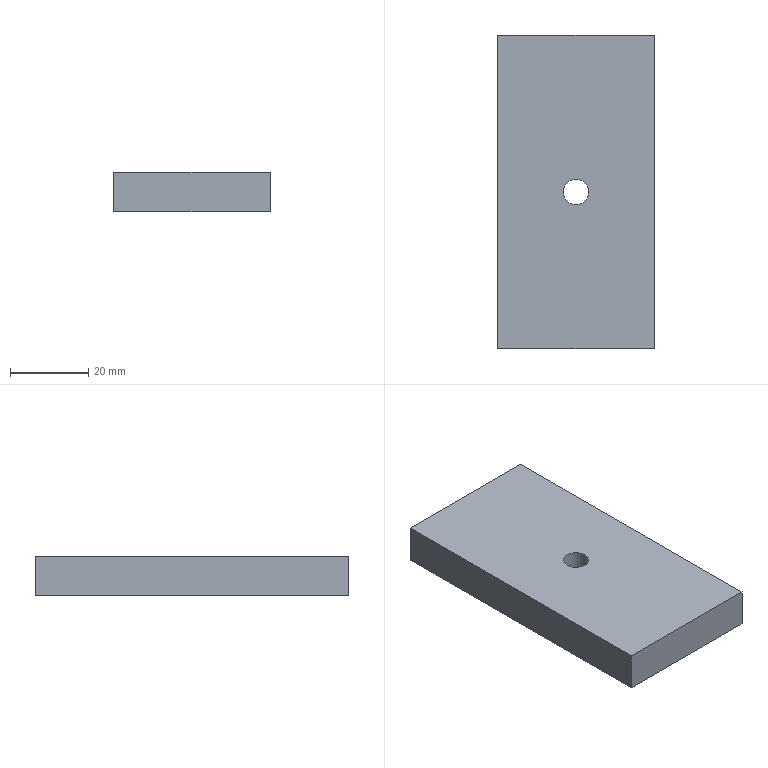Part | STEP file | SynoNew-0304-045 | 1 solid | 7 faces | box 40 x 80 x 10 mm | volume 31668 mm3 | plane 6 | cylinder 1 | commonest cylinder face diameters 6.5 x1
STEP:
#1=CARTESIAN_POINT('',(3.25,0.,10.));
#2=VERTEX_POINT('',#1);
#3=CARTESIAN_POINT('',(-3.25,0.,10.));
#4=VERTEX_POINT('',#3);
#5=CARTESIAN_POINT('',(0.,0.,10.));
#6=DIRECTION('',(0.,0.,-1.));
#7=DIRECTION('',(1.,0.,0.));
#8=AXIS2_PLACEMENT_3D('',#5,#6,#7);
#9=CIRCLE('',#8,3.25);
#10=EDGE_CURVE('',#2,#4,#9,.T.);
#11=ORIENTED_EDGE('',*,*,#10,.F.);
#12=CARTESIAN_POINT('',(0.,0.,10.));
#13=DIRECTION('',(0.,0.,-1.));
#14=DIRECTION('',(1.,0.,0.));
#15=AXIS2_PLACEMENT_3D('',#12,#13,#14);
#16=CIRCLE('',#15,3.25);
#17=EDGE_CURVE('',#4,#2,#16,.T.);
#18=ORIENTED_EDGE('',*,*,#17,.F.);
#19=CARTESIAN_POINT('',(-3.25,0.,0.));
#20=VERTEX_POINT('',#19);
#21=CARTESIAN_POINT('',(-3.25,0.,-80.));
#22=DIRECTION('',(0.,0.,-1.));
#23=VECTOR('',#22,3.25);
#24=LINE('',#21,#23);
#25=EDGE_CURVE('',#4,#20,#24,.T.);
#26=ORIENTED_EDGE('',*,*,#25,.T.);
#27=CARTESIAN_POINT('',(0.,0.,0.));
#28=DIRECTION('',(0.,0.,1.));
#29=DIRECTION('',(1.,0.,0.));
#30=AXIS2_PLACEMENT_3D('',#27,#28,#29);
#31=CIRCLE('',#30,3.25);
#32=EDGE_CURVE('',#20,#20,#31,.T.);
#33=ORIENTED_EDGE('',*,*,#32,.F.);
#34=ORIENTED_EDGE('',*,*,#25,.F.);
#35=EDGE_LOOP('',(#11,#18,#26,#33,#34));
#36=FACE_OUTER_BOUND('',#35,.T.);
#37=CARTESIAN_POINT('',(0.,0.,-80.));
#38=DIRECTION('',(0.,0.,1.));
#39=DIRECTION('',(1.,0.,0.));
#40=AXIS2_PLACEMENT_3D('',#37,#38,#39);
#41=CYLINDRICAL_SURFACE('',#40,3.25);
#42=ADVANCED_FACE('',(#36),#41,.F.);
#43=CARTESIAN_POINT('',(-20.,-40.,0.));
#44=VERTEX_POINT('',#43);
#45=CARTESIAN_POINT('',(20.,-40.,0.));
#46=VERTEX_POINT('',#45);
#47=CARTESIAN_POINT('',(-20.,-40.,0.));
#48=DIRECTION('',(1.,0.,0.));
#49=VECTOR('',#48,10.);
#50=LINE('',#47,#49);
#51=EDGE_CURVE('',#44,#46,#50,.T.);
#52=ORIENTED_EDGE('',*,*,#51,.T.);
#53=CARTESIAN_POINT('',(20.,-40.,10.));
#54=VERTEX_POINT('',#53);
#55=CARTESIAN_POINT('',(20.,-40.,0.));
#56=DIRECTION('',(0.,0.,1.));
#57=VECTOR('',#56,10.);
#58=LINE('',#55,#57);
#59=EDGE_CURVE('',#46,#54,#58,.T.);
#60=ORIENTED_EDGE('',*,*,#59,.T.);
#61=CARTESIAN_POINT('',(-20.,-40.,10.));
#62=VERTEX_POINT('',#61);
#63=CARTESIAN_POINT('',(-20.,-40.,10.));
#64=DIRECTION('',(1.,0.,0.));
#65=VECTOR('',#64,10.);
#66=LINE('',#63,#65);
#67=EDGE_CURVE('',#62,#54,#66,.T.);
#68=ORIENTED_EDGE('',*,*,#67,.F.);
#69=CARTESIAN_POINT('',(-20.,-40.,0.));
#70=DIRECTION('',(0.,0.,1.));
#71=VECTOR('',#70,10.);
#72=LINE('',#69,#71);
#73=EDGE_CURVE('',#44,#62,#72,.T.);
#74=ORIENTED_EDGE('',*,*,#73,.F.);
#75=EDGE_LOOP('',(#52,#60,#68,#74));
#76=FACE_OUTER_BOUND('',#75,.T.);
#77=CARTESIAN_POINT('',(-20.,-40.,0.));
#78=DIRECTION('',(0.,-1.,0.));
#79=DIRECTION('',(1.,0.,0.));
#80=AXIS2_PLACEMENT_3D('',#77,#78,#79);
#81=PLANE('',#80);
#82=ADVANCED_FACE('',(#76),#81,.T.);
#83=CARTESIAN_POINT('',(-20.,40.,0.));
#84=VERTEX_POINT('',#83);
#85=CARTESIAN_POINT('',(-20.,40.,0.));
#86=DIRECTION('',(0.,-1.,0.));
#87=VECTOR('',#86,10.);
#88=LINE('',#85,#87);
#89=EDGE_CURVE('',#84,#44,#88,.T.);
#90=ORIENTED_EDGE('',*,*,#89,.T.);
#91=ORIENTED_EDGE('',*,*,#73,.T.);
#92=CARTESIAN_POINT('',(-20.,40.,10.));
#93=VERTEX_POINT('',#92);
#94=CARTESIAN_POINT('',(-20.,40.,10.));
#95=DIRECTION('',(0.,-1.,0.));
#96=VECTOR('',#95,10.);
#97=LINE('',#94,#96);
#98=EDGE_CURVE('',#93,#62,#97,.T.);
#99=ORIENTED_EDGE('',*,*,#98,.F.);
#100=CARTESIAN_POINT('',(-20.,40.,0.));
#101=DIRECTION('',(0.,0.,1.));
#102=VECTOR('',#101,10.);
#103=LINE('',#100,#102);
#104=EDGE_CURVE('',#84,#93,#103,.T.);
#105=ORIENTED_EDGE('',*,*,#104,.F.);
#106=EDGE_LOOP('',(#90,#91,#99,#105));
#107=FACE_OUTER_BOUND('',#106,.T.);
#108=CARTESIAN_POINT('',(-20.,40.,0.));
#109=DIRECTION('',(-1.,0.,0.));
#110=DIRECTION('',(0.,-1.,0.));
#111=AXIS2_PLACEMENT_3D('',#108,#109,#110);
#112=PLANE('',#111);
#113=ADVANCED_FACE('',(#107),#112,.T.);
#114=CARTESIAN_POINT('',(20.,40.,0.));
#115=VERTEX_POINT('',#114);
#116=CARTESIAN_POINT('',(20.,40.,0.));
#117=DIRECTION('',(-1.,0.,0.));
#118=VECTOR('',#117,10.);
#119=LINE('',#116,#118);
#120=EDGE_CURVE('',#115,#84,#119,.T.);
#121=ORIENTED_EDGE('',*,*,#120,.T.);
#122=ORIENTED_EDGE('',*,*,#104,.T.);
#123=CARTESIAN_POINT('',(20.,40.,10.));
#124=VERTEX_POINT('',#123);
#125=CARTESIAN_POINT('',(20.,40.,10.));
#126=DIRECTION('',(-1.,0.,0.));
#127=VECTOR('',#126,10.);
#128=LINE('',#125,#127);
#129=EDGE_CURVE('',#124,#93,#128,.T.);
#130=ORIENTED_EDGE('',*,*,#129,.F.);
#131=CARTESIAN_POINT('',(20.,40.,0.));
#132=DIRECTION('',(0.,0.,1.));
#133=VECTOR('',#132,10.);
#134=LINE('',#131,#133);
#135=EDGE_CURVE('',#115,#124,#134,.T.);
#136=ORIENTED_EDGE('',*,*,#135,.F.);
#137=EDGE_LOOP('',(#121,#122,#130,#136));
#138=FACE_OUTER_BOUND('',#137,.T.);
#139=CARTESIAN_POINT('',(20.,40.,0.));
#140=DIRECTION('',(0.,1.,0.));
#141=DIRECTION('',(-1.,0.,0.));
#142=AXIS2_PLACEMENT_3D('',#139,#140,#141);
#143=PLANE('',#142);
#144=ADVANCED_FACE('',(#138),#143,.T.);
#145=CARTESIAN_POINT('',(20.,-40.,0.));
#146=DIRECTION('',(0.,1.,0.));
#147=VECTOR('',#146,10.);
#148=LINE('',#145,#147);
#149=EDGE_CURVE('',#46,#115,#148,.T.);
#150=ORIENTED_EDGE('',*,*,#149,.T.);
#151=ORIENTED_EDGE('',*,*,#135,.T.);
#152=CARTESIAN_POINT('',(20.,-40.,10.));
#153=DIRECTION('',(0.,1.,0.));
#154=VECTOR('',#153,10.);
#155=LINE('',#152,#154);
#156=EDGE_CURVE('',#54,#124,#155,.T.);
#157=ORIENTED_EDGE('',*,*,#156,.F.);
#158=ORIENTED_EDGE('',*,*,#59,.F.);
#159=EDGE_LOOP('',(#150,#151,#157,#158));
#160=FACE_OUTER_BOUND('',#159,.T.);
#161=CARTESIAN_POINT('',(20.,-40.,0.));
#162=DIRECTION('',(1.,0.,0.));
#163=DIRECTION('',(0.,1.,0.));
#164=AXIS2_PLACEMENT_3D('',#161,#162,#163);
#165=PLANE('',#164);
#166=ADVANCED_FACE('',(#160),#165,.T.);
#167=ORIENTED_EDGE('',*,*,#156,.T.);
#168=ORIENTED_EDGE('',*,*,#129,.T.);
#169=ORIENTED_EDGE('',*,*,#98,.T.);
#170=ORIENTED_EDGE('',*,*,#67,.T.);
#171=EDGE_LOOP('',(#167,#168,#169,#170));
#172=FACE_OUTER_BOUND('',#171,.T.);
#173=ORIENTED_EDGE('',*,*,#10,.T.);
#174=ORIENTED_EDGE('',*,*,#17,.T.);
#175=EDGE_LOOP('',(#173,#174));
#176=FACE_BOUND('',#175,.T.);
#177=CARTESIAN_POINT('',(0.,0.,10.));
#178=DIRECTION('',(0.,0.,1.));
#179=DIRECTION('',(1.,0.,0.));
#180=AXIS2_PLACEMENT_3D('',#177,#178,#179);
#181=PLANE('',#180);
#182=ADVANCED_FACE('',(#172,#176),#181,.T.);
#183=ORIENTED_EDGE('',*,*,#149,.F.);
#184=ORIENTED_EDGE('',*,*,#51,.F.);
#185=ORIENTED_EDGE('',*,*,#89,.F.);
#186=ORIENTED_EDGE('',*,*,#120,.F.);
#187=EDGE_LOOP('',(#183,#184,#185,#186));
#188=FACE_OUTER_BOUND('',#187,.T.);
#189=ORIENTED_EDGE('',*,*,#32,.T.);
#190=EDGE_LOOP('',(#189));
#191=FACE_BOUND('',#190,.T.);
#192=CARTESIAN_POINT('',(0.,0.,0.));
#193=DIRECTION('',(0.,0.,1.));
#194=DIRECTION('',(1.,0.,0.));
#195=AXIS2_PLACEMENT_3D('',#192,#193,#194);
#196=PLANE('',#195);
#197=ADVANCED_FACE('',(#188,#191),#196,.F.);
#198=CLOSED_SHELL('',(#42,#82,#113,#144,#166,#182,#197));
#199=MANIFOLD_SOLID_BREP('',#198);
#200=(LENGTH_UNIT()NAMED_UNIT(*)SI_UNIT(.MILLI.,.METRE.));
#201=UNCERTAINTY_MEASURE_WITH_UNIT(LENGTH_MEASURE(0.01),#200,'','');
#202=(NAMED_UNIT(*)PLANE_ANGLE_UNIT()SI_UNIT($,.RADIAN.));
#203=(NAMED_UNIT(*)SI_UNIT($,.STERADIAN.)SOLID_ANGLE_UNIT());
#204=(GEOMETRIC_REPRESENTATION_CONTEXT(3)GLOBAL_UNCERTAINTY_ASSIGNED_CONTEXT((#201))GLOBAL_UNIT_ASSIGNED_CONTEXT((#200,#202,#203))REPRESENTATION_CONTEXT('',''));
#205=ADVANCED_BREP_SHAPE_REPRESENTATION('',(#199),#204);